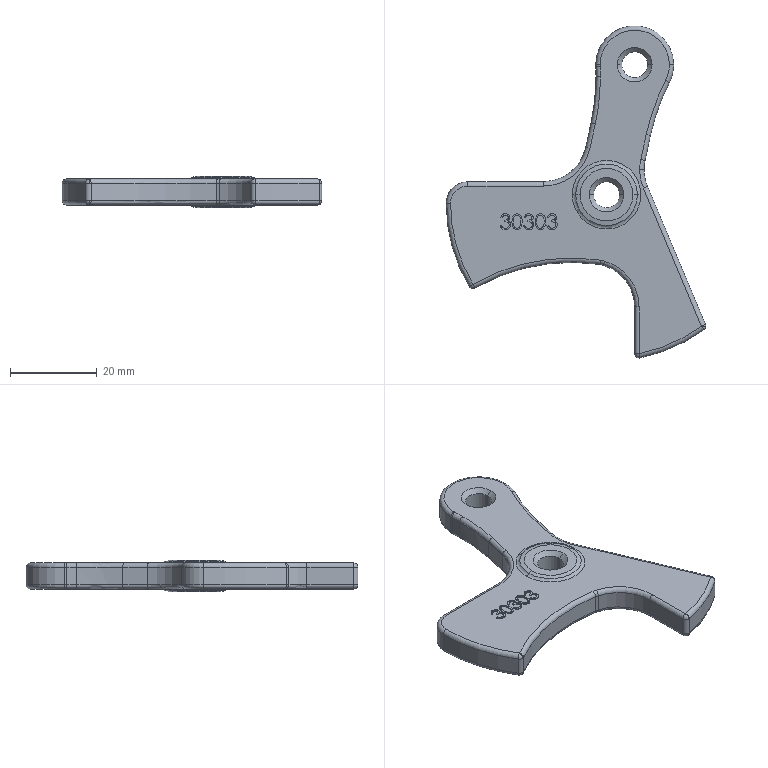Part | STEP file | 101000005924 | 1 solid | 303 faces | box 59.899 x 76.667 x 7.2 mm | volume 10614 mm3 | plane 123 | spline 77 | cylinder 45 | torus 34 | cone 12 | sphere 12 | commonest cylinder face diameters 2 x14 6 x4 20 x4 18 x3 100 x3 0.204 x2